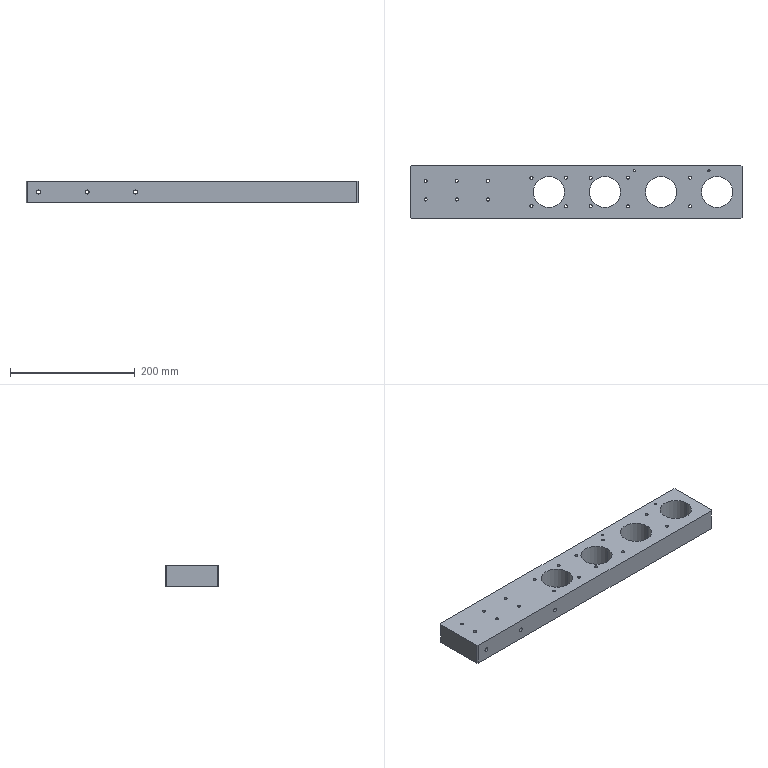Part | STEP file | X-axis mounting plate | 1 solid | 81 faces | box 533 x 86 x 35 mm | volume 1297130 mm3 | cylinder 62 | plane 13 | cone 6 | commonest cylinder face diameters 5 x36 50 x8 3.3 x6 6.6 x6 11 x6